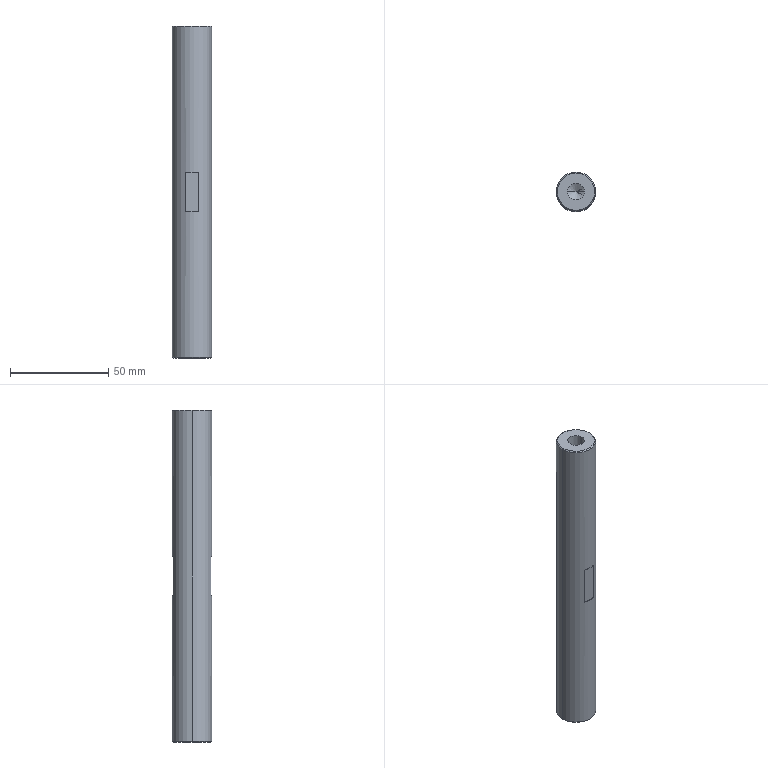Part | STEP file | 11-FG-Z01011 | 1 solid | 22 faces | box 20 x 20 x 169 mm | volume 50117 mm3 | cone 8 | plane 8 | cylinder 6 | commonest cylinder face diameters 8.5 x4 20 x2
STEP:
#1=CARTESIAN_POINT('',(-9.5,0.,0.));
#2=VERTEX_POINT('',#1);
#3=CARTESIAN_POINT('',(9.5,0.,0.));
#4=VERTEX_POINT('',#3);
#5=CARTESIAN_POINT('',(0.,0.,0.));
#6=DIRECTION('',(0.,0.,-1.));
#7=DIRECTION('',(1.,0.,0.));
#8=AXIS2_PLACEMENT_3D('',#5,#6,#7);
#9=CIRCLE('',#8,9.5);
#10=EDGE_CURVE('',#2,#4,#9,.T.);
#11=ORIENTED_EDGE('',*,*,#10,.F.);
#12=CARTESIAN_POINT('',(-10.,0.,0.5));
#13=VERTEX_POINT('',#12);
#14=CARTESIAN_POINT('',(-10.,0.,0.5));
#15=DIRECTION('',(-0.7071,0.,0.7071));
#16=VECTOR('',#15,1000.);
#17=LINE('',#14,#16);
#18=EDGE_CURVE('',#2,#13,#17,.T.);
#19=ORIENTED_EDGE('',*,*,#18,.T.);
#20=CARTESIAN_POINT('',(10.,0.,0.5));
#21=VERTEX_POINT('',#20);
#22=CARTESIAN_POINT('',(0.,0.,0.5));
#23=DIRECTION('',(0.,0.,1.));
#24=DIRECTION('',(1.,0.,0.));
#25=AXIS2_PLACEMENT_3D('',#22,#23,#24);
#26=CIRCLE('',#25,10.);
#27=EDGE_CURVE('',#21,#13,#26,.T.);
#28=ORIENTED_EDGE('',*,*,#27,.F.);
#29=CARTESIAN_POINT('',(10.,0.,0.5));
#30=DIRECTION('',(0.7071,0.,0.7071));
#31=VECTOR('',#30,1000.);
#32=LINE('',#29,#31);
#33=EDGE_CURVE('',#4,#21,#32,.T.);
#34=ORIENTED_EDGE('',*,*,#33,.F.);
#35=EDGE_LOOP('',(#11,#19,#28,#34));
#36=FACE_OUTER_BOUND('',#35,.T.);
#37=CARTESIAN_POINT('',(0.,0.,0.5));
#38=DIRECTION('',(0.,0.,1.));
#39=DIRECTION('',(1.,0.,0.));
#40=AXIS2_PLACEMENT_3D('',#37,#38,#39);
#41=CONICAL_SURFACE('',#40,10.,0.7854);
#42=ADVANCED_FACE('',(#36),#41,.T.);
#43=CARTESIAN_POINT('',(9.5,0.,169.));
#44=VERTEX_POINT('',#43);
#45=CARTESIAN_POINT('',(-9.5,0.,169.));
#46=VERTEX_POINT('',#45);
#47=CARTESIAN_POINT('',(0.,0.,169.));
#48=DIRECTION('',(0.,0.,1.));
#49=DIRECTION('',(1.,0.,0.));
#50=AXIS2_PLACEMENT_3D('',#47,#48,#49);
#51=CIRCLE('',#50,9.5);
#52=EDGE_CURVE('',#44,#46,#51,.T.);
#53=ORIENTED_EDGE('',*,*,#52,.F.);
#54=CARTESIAN_POINT('',(10.,0.,168.5));
#55=VERTEX_POINT('',#54);
#56=CARTESIAN_POINT('',(9.5,0.,169.));
#57=DIRECTION('',(0.7071,0.,-0.7071));
#58=VECTOR('',#57,1000.);
#59=LINE('',#56,#58);
#60=EDGE_CURVE('',#44,#55,#59,.T.);
#61=ORIENTED_EDGE('',*,*,#60,.T.);
#62=CARTESIAN_POINT('',(-10.,0.,168.5));
#63=VERTEX_POINT('',#62);
#64=CARTESIAN_POINT('',(0.,0.,168.5));
#65=DIRECTION('',(0.,0.,-1.));
#66=DIRECTION('',(1.,0.,0.));
#67=AXIS2_PLACEMENT_3D('',#64,#65,#66);
#68=CIRCLE('',#67,10.);
#69=EDGE_CURVE('',#63,#55,#68,.T.);
#70=ORIENTED_EDGE('',*,*,#69,.F.);
#71=CARTESIAN_POINT('',(-9.5,0.,169.));
#72=DIRECTION('',(-0.7071,0.,-0.7071));
#73=VECTOR('',#72,1000.);
#74=LINE('',#71,#73);
#75=EDGE_CURVE('',#46,#63,#74,.T.);
#76=ORIENTED_EDGE('',*,*,#75,.F.);
#77=EDGE_LOOP('',(#53,#61,#70,#76));
#78=FACE_OUTER_BOUND('',#77,.T.);
#79=CARTESIAN_POINT('',(0.,0.,169.));
#80=DIRECTION('',(0.,0.,-1.));
#81=DIRECTION('',(-1.,0.,0.));
#82=AXIS2_PLACEMENT_3D('',#79,#80,#81);
#83=CONICAL_SURFACE('',#82,9.5,0.7854);
#84=ADVANCED_FACE('',(#78),#83,.T.);
#85=CARTESIAN_POINT('',(4.25,0.,24.5));
#86=VERTEX_POINT('',#85);
#87=CARTESIAN_POINT('',(-4.25,0.,24.5));
#88=VERTEX_POINT('',#87);
#89=CARTESIAN_POINT('',(0.,0.,24.5));
#90=DIRECTION('',(0.,0.,-1.));
#91=DIRECTION('',(-1.,0.,0.));
#92=AXIS2_PLACEMENT_3D('',#89,#90,#91);
#93=CIRCLE('',#92,4.25);
#94=EDGE_CURVE('',#86,#88,#93,.T.);
#95=ORIENTED_EDGE('',*,*,#94,.F.);
#96=CARTESIAN_POINT('',(4.25,0.,0.));
#97=VERTEX_POINT('',#96);
#98=CARTESIAN_POINT('',(4.25,0.,0.));
#99=DIRECTION('',(0.,0.,-1.));
#100=VECTOR('',#99,1000.);
#101=LINE('',#98,#100);
#102=EDGE_CURVE('',#86,#97,#101,.T.);
#103=ORIENTED_EDGE('',*,*,#102,.T.);
#104=CARTESIAN_POINT('',(-4.25,0.,0.));
#105=VERTEX_POINT('',#104);
#106=CARTESIAN_POINT('',(0.,0.,0.));
#107=DIRECTION('',(0.,0.,-1.));
#108=DIRECTION('',(-1.,0.,0.));
#109=AXIS2_PLACEMENT_3D('',#106,#107,#108);
#110=CIRCLE('',#109,4.25);
#111=EDGE_CURVE('',#97,#105,#110,.T.);
#112=ORIENTED_EDGE('',*,*,#111,.T.);
#113=CARTESIAN_POINT('',(-4.25,0.,0.));
#114=DIRECTION('',(0.,0.,-1.));
#115=VECTOR('',#114,1000.);
#116=LINE('',#113,#115);
#117=EDGE_CURVE('',#88,#105,#116,.T.);
#118=ORIENTED_EDGE('',*,*,#117,.F.);
#119=EDGE_LOOP('',(#95,#103,#112,#118));
#120=FACE_OUTER_BOUND('',#119,.T.);
#121=CARTESIAN_POINT('',(0.,0.,0.));
#122=DIRECTION('',(0.,0.,-1.));
#123=DIRECTION('',(-1.,0.,0.));
#124=AXIS2_PLACEMENT_3D('',#121,#122,#123);
#125=CYLINDRICAL_SURFACE('',#124,4.25);
#126=ADVANCED_FACE('',(#120),#125,.F.);
#127=CARTESIAN_POINT('',(0.,0.,27.054));
#128=VERTEX_POINT('',#127);
#129=CARTESIAN_POINT('',(-4.25,0.,24.5));
#130=DIRECTION('',(-0.8572,0.,-0.515));
#131=VECTOR('',#130,1000.);
#132=LINE('',#129,#131);
#133=EDGE_CURVE('',#128,#88,#132,.T.);
#134=ORIENTED_EDGE('',*,*,#133,.F.);
#135=CARTESIAN_POINT('',(4.25,0.,24.5));
#136=DIRECTION('',(0.8572,0.,-0.515));
#137=VECTOR('',#136,1000.);
#138=LINE('',#135,#137);
#139=EDGE_CURVE('',#128,#86,#138,.T.);
#140=ORIENTED_EDGE('',*,*,#139,.T.);
#141=ORIENTED_EDGE('',*,*,#94,.T.);
#142=EDGE_LOOP('',(#134,#140,#141));
#143=FACE_OUTER_BOUND('',#142,.T.);
#144=CARTESIAN_POINT('',(0.,0.,24.5));
#145=DIRECTION('',(0.,0.,-1.));
#146=DIRECTION('',(-1.,0.,0.));
#147=AXIS2_PLACEMENT_3D('',#144,#145,#146);
#148=CONICAL_SURFACE('',#147,4.25,1.03);
#149=ADVANCED_FACE('',(#143),#148,.F.);
#150=CARTESIAN_POINT('',(-4.25,0.,144.5));
#151=VERTEX_POINT('',#150);
#152=CARTESIAN_POINT('',(4.25,0.,144.5));
#153=VERTEX_POINT('',#152);
#154=CARTESIAN_POINT('',(0.,0.,144.5));
#155=DIRECTION('',(0.,0.,1.));
#156=DIRECTION('',(1.,0.,0.));
#157=AXIS2_PLACEMENT_3D('',#154,#155,#156);
#158=CIRCLE('',#157,4.25);
#159=EDGE_CURVE('',#151,#153,#158,.T.);
#160=ORIENTED_EDGE('',*,*,#159,.F.);
#161=CARTESIAN_POINT('',(-4.25,0.,169.));
#162=VERTEX_POINT('',#161);
#163=CARTESIAN_POINT('',(-4.25,0.,169.));
#164=DIRECTION('',(0.,0.,1.));
#165=VECTOR('',#164,1000.);
#166=LINE('',#163,#165);
#167=EDGE_CURVE('',#151,#162,#166,.T.);
#168=ORIENTED_EDGE('',*,*,#167,.T.);
#169=CARTESIAN_POINT('',(4.25,0.,169.));
#170=VERTEX_POINT('',#169);
#171=CARTESIAN_POINT('',(0.,0.,169.));
#172=DIRECTION('',(0.,0.,1.));
#173=DIRECTION('',(1.,0.,0.));
#174=AXIS2_PLACEMENT_3D('',#171,#172,#173);
#175=CIRCLE('',#174,4.25);
#176=EDGE_CURVE('',#162,#170,#175,.T.);
#177=ORIENTED_EDGE('',*,*,#176,.T.);
#178=CARTESIAN_POINT('',(4.25,0.,169.));
#179=DIRECTION('',(0.,0.,1.));
#180=VECTOR('',#179,1000.);
#181=LINE('',#178,#180);
#182=EDGE_CURVE('',#153,#170,#181,.T.);
#183=ORIENTED_EDGE('',*,*,#182,.F.);
#184=EDGE_LOOP('',(#160,#168,#177,#183));
#185=FACE_OUTER_BOUND('',#184,.T.);
#186=CARTESIAN_POINT('',(0.,0.,169.));
#187=DIRECTION('',(0.,0.,1.));
#188=DIRECTION('',(1.,0.,0.));
#189=AXIS2_PLACEMENT_3D('',#186,#187,#188);
#190=CYLINDRICAL_SURFACE('',#189,4.25);
#191=ADVANCED_FACE('',(#185),#190,.F.);
#192=CARTESIAN_POINT('',(0.,0.,141.946));
#193=VERTEX_POINT('',#192);
#194=CARTESIAN_POINT('',(4.25,0.,144.5));
#195=DIRECTION('',(0.8572,0.,0.515));
#196=VECTOR('',#195,1000.);
#197=LINE('',#194,#196);
#198=EDGE_CURVE('',#193,#153,#197,.T.);
#199=ORIENTED_EDGE('',*,*,#198,.F.);
#200=CARTESIAN_POINT('',(-4.25,0.,144.5));
#201=DIRECTION('',(-0.8572,0.,0.515));
#202=VECTOR('',#201,1000.);
#203=LINE('',#200,#202);
#204=EDGE_CURVE('',#193,#151,#203,.T.);
#205=ORIENTED_EDGE('',*,*,#204,.T.);
#206=ORIENTED_EDGE('',*,*,#159,.T.);
#207=EDGE_LOOP('',(#199,#205,#206));
#208=FACE_OUTER_BOUND('',#207,.T.);
#209=CARTESIAN_POINT('',(0.,0.,144.5));
#210=DIRECTION('',(0.,0.,1.));
#211=DIRECTION('',(1.,0.,0.));
#212=AXIS2_PLACEMENT_3D('',#209,#210,#211);
#213=CONICAL_SURFACE('',#212,4.25,1.03);
#214=ADVANCED_FACE('',(#208),#213,.F.);
#215=CARTESIAN_POINT('',(-3.122,9.5,94.5));
#216=VERTEX_POINT('',#215);
#217=CARTESIAN_POINT('',(3.122,9.5,94.5));
#218=VERTEX_POINT('',#217);
#219=CARTESIAN_POINT('',(0.,0.,94.5));
#220=DIRECTION('',(0.,0.,-1.));
#221=DIRECTION('',(-1.,0.,0.));
#222=AXIS2_PLACEMENT_3D('',#219,#220,#221);
#223=CIRCLE('',#222,10.);
#224=EDGE_CURVE('',#216,#218,#223,.T.);
#225=ORIENTED_EDGE('',*,*,#224,.F.);
#226=CARTESIAN_POINT('',(-3.122,9.5,74.5));
#227=VERTEX_POINT('',#226);
#228=CARTESIAN_POINT('',(-3.122,9.5,169.));
#229=DIRECTION('',(0.,0.,-1.));
#230=VECTOR('',#229,1000.);
#231=LINE('',#228,#230);
#232=EDGE_CURVE('',#216,#227,#231,.T.);
#233=ORIENTED_EDGE('',*,*,#232,.T.);
#234=CARTESIAN_POINT('',(3.122,9.5,74.5));
#235=VERTEX_POINT('',#234);
#236=CARTESIAN_POINT('',(0.,0.,74.5));
#237=DIRECTION('',(0.,0.,-1.));
#238=DIRECTION('',(-1.,0.,0.));
#239=AXIS2_PLACEMENT_3D('',#236,#237,#238);
#240=CIRCLE('',#239,10.);
#241=EDGE_CURVE('',#227,#235,#240,.T.);
#242=ORIENTED_EDGE('',*,*,#241,.T.);
#243=CARTESIAN_POINT('',(3.122,9.5,169.));
#244=DIRECTION('',(0.,0.,1.));
#245=VECTOR('',#244,1000.);
#246=LINE('',#243,#245);
#247=EDGE_CURVE('',#235,#218,#246,.T.);
#248=ORIENTED_EDGE('',*,*,#247,.T.);
#249=EDGE_LOOP('',(#225,#233,#242,#248));
#250=FACE_BOUND('',#249,.T.);
#251=ORIENTED_EDGE('',*,*,#69,.T.);
#252=CARTESIAN_POINT('',(10.,0.,169.));
#253=DIRECTION('',(0.,0.,-1.));
#254=VECTOR('',#253,1000.);
#255=LINE('',#252,#254);
#256=EDGE_CURVE('',#55,#21,#255,.T.);
#257=ORIENTED_EDGE('',*,*,#256,.T.);
#258=ORIENTED_EDGE('',*,*,#27,.T.);
#259=CARTESIAN_POINT('',(-10.,0.,169.));
#260=DIRECTION('',(0.,0.,-1.));
#261=VECTOR('',#260,1000.);
#262=LINE('',#259,#261);
#263=EDGE_CURVE('',#63,#13,#262,.T.);
#264=ORIENTED_EDGE('',*,*,#263,.F.);
#265=EDGE_LOOP('',(#251,#257,#258,#264));
#266=FACE_OUTER_BOUND('',#265,.T.);
#267=CARTESIAN_POINT('',(0.,0.,169.));
#268=DIRECTION('',(0.,0.,-1.));
#269=DIRECTION('',(-1.,0.,0.));
#270=AXIS2_PLACEMENT_3D('',#267,#268,#269);
#271=CYLINDRICAL_SURFACE('',#270,10.);
#272=ADVANCED_FACE('',(#250,#266),#271,.T.);
#273=ORIENTED_EDGE('',*,*,#256,.F.);
#274=CARTESIAN_POINT('',(0.,0.,168.5));
#275=DIRECTION('',(0.,0.,-1.));
#276=DIRECTION('',(1.,0.,0.));
#277=AXIS2_PLACEMENT_3D('',#274,#275,#276);
#278=CIRCLE('',#277,10.);
#279=EDGE_CURVE('',#55,#63,#278,.T.);
#280=ORIENTED_EDGE('',*,*,#279,.T.);
#281=ORIENTED_EDGE('',*,*,#263,.T.);
#282=CARTESIAN_POINT('',(0.,0.,0.5));
#283=DIRECTION('',(0.,0.,1.));
#284=DIRECTION('',(1.,0.,0.));
#285=AXIS2_PLACEMENT_3D('',#282,#283,#284);
#286=CIRCLE('',#285,10.);
#287=EDGE_CURVE('',#13,#21,#286,.T.);
#288=ORIENTED_EDGE('',*,*,#287,.T.);
#289=EDGE_LOOP('',(#273,#280,#281,#288));
#290=FACE_OUTER_BOUND('',#289,.T.);
#291=CARTESIAN_POINT('',(3.122,-9.5,94.5));
#292=VERTEX_POINT('',#291);
#293=CARTESIAN_POINT('',(-3.122,-9.5,94.5));
#294=VERTEX_POINT('',#293);
#295=CARTESIAN_POINT('',(0.,0.,94.5));
#296=DIRECTION('',(0.,0.,-1.));
#297=DIRECTION('',(-1.,0.,0.));
#298=AXIS2_PLACEMENT_3D('',#295,#296,#297);
#299=CIRCLE('',#298,10.);
#300=EDGE_CURVE('',#292,#294,#299,.T.);
#301=ORIENTED_EDGE('',*,*,#300,.F.);
#302=CARTESIAN_POINT('',(3.122,-9.5,74.5));
#303=VERTEX_POINT('',#302);
#304=CARTESIAN_POINT('',(3.122,-9.5,169.));
#305=DIRECTION('',(0.,0.,-1.));
#306=VECTOR('',#305,1000.);
#307=LINE('',#304,#306);
#308=EDGE_CURVE('',#292,#303,#307,.T.);
#309=ORIENTED_EDGE('',*,*,#308,.T.);
#310=CARTESIAN_POINT('',(-3.122,-9.5,74.5));
#311=VERTEX_POINT('',#310);
#312=CARTESIAN_POINT('',(0.,0.,74.5));
#313=DIRECTION('',(0.,0.,-1.));
#314=DIRECTION('',(-1.,0.,0.));
#315=AXIS2_PLACEMENT_3D('',#312,#313,#314);
#316=CIRCLE('',#315,10.);
#317=EDGE_CURVE('',#303,#311,#316,.T.);
#318=ORIENTED_EDGE('',*,*,#317,.T.);
#319=CARTESIAN_POINT('',(-3.122,-9.5,169.));
#320=DIRECTION('',(0.,0.,1.));
#321=VECTOR('',#320,1000.);
#322=LINE('',#319,#321);
#323=EDGE_CURVE('',#311,#294,#322,.T.);
#324=ORIENTED_EDGE('',*,*,#323,.T.);
#325=EDGE_LOOP('',(#301,#309,#318,#324));
#326=FACE_BOUND('',#325,.T.);
#327=CARTESIAN_POINT('',(0.,0.,169.));
#328=DIRECTION('',(0.,0.,-1.));
#329=DIRECTION('',(-1.,0.,0.));
#330=AXIS2_PLACEMENT_3D('',#327,#328,#329);
#331=CYLINDRICAL_SURFACE('',#330,10.);
#332=ADVANCED_FACE('',(#290,#326),#331,.T.);
#333=CARTESIAN_POINT('',(0.,0.,169.));
#334=DIRECTION('',(0.,0.,1.));
#335=DIRECTION('',(1.,0.,0.));
#336=AXIS2_PLACEMENT_3D('',#333,#334,#335);
#337=CIRCLE('',#336,9.5);
#338=EDGE_CURVE('',#46,#44,#337,.T.);
#339=ORIENTED_EDGE('',*,*,#338,.T.);
#340=ORIENTED_EDGE('',*,*,#52,.T.);
#341=EDGE_LOOP('',(#339,#340));
#342=FACE_OUTER_BOUND('',#341,.T.);
#343=CARTESIAN_POINT('',(0.,0.,169.));
#344=DIRECTION('',(0.,0.,1.));
#345=DIRECTION('',(1.,0.,0.));
#346=AXIS2_PLACEMENT_3D('',#343,#344,#345);
#347=CIRCLE('',#346,4.25);
#348=EDGE_CURVE('',#170,#162,#347,.T.);
#349=ORIENTED_EDGE('',*,*,#348,.F.);
#350=ORIENTED_EDGE('',*,*,#176,.F.);
#351=EDGE_LOOP('',(#349,#350));
#352=FACE_BOUND('',#351,.T.);
#353=CARTESIAN_POINT('',(0.,0.,169.));
#354=DIRECTION('',(0.,0.,1.));
#355=DIRECTION('',(1.,0.,0.));
#356=AXIS2_PLACEMENT_3D('',#353,#354,#355);
#357=PLANE('',#356);
#358=ADVANCED_FACE('',(#342,#352),#357,.T.);
#359=CARTESIAN_POINT('',(0.,0.,0.));
#360=DIRECTION('',(0.,0.,-1.));
#361=DIRECTION('',(1.,0.,0.));
#362=AXIS2_PLACEMENT_3D('',#359,#360,#361);
#363=CIRCLE('',#362,9.5);
#364=EDGE_CURVE('',#4,#2,#363,.T.);
#365=ORIENTED_EDGE('',*,*,#364,.T.);
#366=ORIENTED_EDGE('',*,*,#10,.T.);
#367=EDGE_LOOP('',(#365,#366));
#368=FACE_OUTER_BOUND('',#367,.T.);
#369=CARTESIAN_POINT('',(0.,0.,0.));
#370=DIRECTION('',(0.,0.,-1.));
#371=DIRECTION('',(-1.,0.,0.));
#372=AXIS2_PLACEMENT_3D('',#369,#370,#371);
#373=CIRCLE('',#372,4.25);
#374=EDGE_CURVE('',#105,#97,#373,.T.);
#375=ORIENTED_EDGE('',*,*,#374,.F.);
#376=ORIENTED_EDGE('',*,*,#111,.F.);
#377=EDGE_LOOP('',(#375,#376));
#378=FACE_BOUND('',#377,.T.);
#379=CARTESIAN_POINT('',(0.,0.,0.));
#380=DIRECTION('',(0.,0.,1.));
#381=DIRECTION('',(1.,0.,0.));
#382=AXIS2_PLACEMENT_3D('',#379,#380,#381);
#383=PLANE('',#382);
#384=ADVANCED_FACE('',(#368,#378),#383,.F.);
#385=ORIENTED_EDGE('',*,*,#204,.F.);
#386=ORIENTED_EDGE('',*,*,#198,.T.);
#387=CARTESIAN_POINT('',(0.,0.,144.5));
#388=DIRECTION('',(0.,0.,1.));
#389=DIRECTION('',(1.,0.,0.));
#390=AXIS2_PLACEMENT_3D('',#387,#388,#389);
#391=CIRCLE('',#390,4.25);
#392=EDGE_CURVE('',#153,#151,#391,.T.);
#393=ORIENTED_EDGE('',*,*,#392,.T.);
#394=EDGE_LOOP('',(#385,#386,#393));
#395=FACE_OUTER_BOUND('',#394,.T.);
#396=CARTESIAN_POINT('',(0.,0.,144.5));
#397=DIRECTION('',(0.,0.,1.));
#398=DIRECTION('',(1.,0.,0.));
#399=AXIS2_PLACEMENT_3D('',#396,#397,#398);
#400=CONICAL_SURFACE('',#399,4.25,1.03);
#401=ADVANCED_FACE('',(#395),#400,.F.);
#402=ORIENTED_EDGE('',*,*,#167,.F.);
#403=ORIENTED_EDGE('',*,*,#392,.F.);
#404=ORIENTED_EDGE('',*,*,#182,.T.);
#405=ORIENTED_EDGE('',*,*,#348,.T.);
#406=EDGE_LOOP('',(#402,#403,#404,#405));
#407=FACE_OUTER_BOUND('',#406,.T.);
#408=CARTESIAN_POINT('',(0.,0.,169.));
#409=DIRECTION('',(0.,0.,1.));
#410=DIRECTION('',(1.,0.,0.));
#411=AXIS2_PLACEMENT_3D('',#408,#409,#410);
#412=CYLINDRICAL_SURFACE('',#411,4.25);
#413=ADVANCED_FACE('',(#407),#412,.F.);
#414=ORIENTED_EDGE('',*,*,#139,.F.);
#415=ORIENTED_EDGE('',*,*,#133,.T.);
#416=CARTESIAN_POINT('',(0.,0.,24.5));
#417=DIRECTION('',(0.,0.,-1.));
#418=DIRECTION('',(-1.,0.,0.));
#419=AXIS2_PLACEMENT_3D('',#416,#417,#418);
#420=CIRCLE('',#419,4.25);
#421=EDGE_CURVE('',#88,#86,#420,.T.);
#422=ORIENTED_EDGE('',*,*,#421,.T.);
#423=EDGE_LOOP('',(#414,#415,#422));
#424=FACE_OUTER_BOUND('',#423,.T.);
#425=CARTESIAN_POINT('',(0.,0.,24.5));
#426=DIRECTION('',(0.,0.,-1.));
#427=DIRECTION('',(-1.,0.,0.));
#428=AXIS2_PLACEMENT_3D('',#425,#426,#427);
#429=CONICAL_SURFACE('',#428,4.25,1.03);
#430=ADVANCED_FACE('',(#424),#429,.F.);
#431=ORIENTED_EDGE('',*,*,#102,.F.);
#432=ORIENTED_EDGE('',*,*,#421,.F.);
#433=ORIENTED_EDGE('',*,*,#117,.T.);
#434=ORIENTED_EDGE('',*,*,#374,.T.);
#435=EDGE_LOOP('',(#431,#432,#433,#434));
#436=FACE_OUTER_BOUND('',#435,.T.);
#437=CARTESIAN_POINT('',(0.,0.,0.));
#438=DIRECTION('',(0.,0.,-1.));
#439=DIRECTION('',(-1.,0.,0.));
#440=AXIS2_PLACEMENT_3D('',#437,#438,#439);
#441=CYLINDRICAL_SURFACE('',#440,4.25);
#442=ADVANCED_FACE('',(#436),#441,.F.);
#443=ORIENTED_EDGE('',*,*,#60,.F.);
#444=ORIENTED_EDGE('',*,*,#338,.F.);
#445=ORIENTED_EDGE('',*,*,#75,.T.);
#446=ORIENTED_EDGE('',*,*,#279,.F.);
#447=EDGE_LOOP('',(#443,#444,#445,#446));
#448=FACE_OUTER_BOUND('',#447,.T.);
#449=CARTESIAN_POINT('',(0.,0.,169.));
#450=DIRECTION('',(0.,0.,-1.));
#451=DIRECTION('',(-1.,0.,0.));
#452=AXIS2_PLACEMENT_3D('',#449,#450,#451);
#453=CONICAL_SURFACE('',#452,9.5,0.7854);
#454=ADVANCED_FACE('',(#448),#453,.T.);
#455=ORIENTED_EDGE('',*,*,#18,.F.);
#456=ORIENTED_EDGE('',*,*,#364,.F.);
#457=ORIENTED_EDGE('',*,*,#33,.T.);
#458=ORIENTED_EDGE('',*,*,#287,.F.);
#459=EDGE_LOOP('',(#455,#456,#457,#458));
#460=FACE_OUTER_BOUND('',#459,.T.);
#461=CARTESIAN_POINT('',(0.,0.,0.5));
#462=DIRECTION('',(0.,0.,1.));
#463=DIRECTION('',(1.,0.,0.));
#464=AXIS2_PLACEMENT_3D('',#461,#462,#463);
#465=CONICAL_SURFACE('',#464,10.,0.7854);
#466=ADVANCED_FACE('',(#460),#465,.T.);
#467=CARTESIAN_POINT('',(4.899,9.5,94.5));
#468=DIRECTION('',(-1.,0.,0.));
#469=VECTOR('',#468,1000.);
#470=LINE('',#467,#469);
#471=EDGE_CURVE('',#218,#216,#470,.T.);
#472=ORIENTED_EDGE('',*,*,#471,.F.);
#473=ORIENTED_EDGE('',*,*,#247,.F.);
#474=CARTESIAN_POINT('',(4.899,9.5,74.5));
#475=DIRECTION('',(-1.,0.,0.));
#476=VECTOR('',#475,1000.);
#477=LINE('',#474,#476);
#478=EDGE_CURVE('',#235,#227,#477,.T.);
#479=ORIENTED_EDGE('',*,*,#478,.T.);
#480=ORIENTED_EDGE('',*,*,#232,.F.);
#481=EDGE_LOOP('',(#472,#473,#479,#480));
#482=FACE_OUTER_BOUND('',#481,.T.);
#483=CARTESIAN_POINT('',(4.899,9.5,94.5));
#484=DIRECTION('',(0.,-1.,0.));
#485=DIRECTION('',(0.,0.,-1.));
#486=AXIS2_PLACEMENT_3D('',#483,#484,#485);
#487=PLANE('',#486);
#488=ADVANCED_FACE('',(#482),#487,.F.);
#489=ORIENTED_EDGE('',*,*,#224,.T.);
#490=ORIENTED_EDGE('',*,*,#471,.T.);
#491=EDGE_LOOP('',(#489,#490));
#492=FACE_OUTER_BOUND('',#491,.T.);
#493=CARTESIAN_POINT('',(0.,0.,94.5));
#494=DIRECTION('',(0.,0.,-1.));
#495=DIRECTION('',(-1.,0.,0.));
#496=AXIS2_PLACEMENT_3D('',#493,#494,#495);
#497=PLANE('',#496);
#498=ADVANCED_FACE('',(#492),#497,.T.);
#499=ORIENTED_EDGE('',*,*,#478,.F.);
#500=ORIENTED_EDGE('',*,*,#241,.F.);
#501=EDGE_LOOP('',(#499,#500));
#502=FACE_OUTER_BOUND('',#501,.T.);
#503=CARTESIAN_POINT('',(0.,0.,74.5));
#504=DIRECTION('',(0.,0.,-1.));
#505=DIRECTION('',(-1.,0.,0.));
#506=AXIS2_PLACEMENT_3D('',#503,#504,#505);
#507=PLANE('',#506);
#508=ADVANCED_FACE('',(#502),#507,.F.);
#509=CARTESIAN_POINT('',(4.899,-9.5,94.5));
#510=DIRECTION('',(1.,0.,0.));
#511=VECTOR('',#510,1000.);
#512=LINE('',#509,#511);
#513=EDGE_CURVE('',#294,#292,#512,.T.);
#514=ORIENTED_EDGE('',*,*,#513,.F.);
#515=ORIENTED_EDGE('',*,*,#323,.F.);
#516=CARTESIAN_POINT('',(4.899,-9.5,74.5));
#517=DIRECTION('',(1.,0.,0.));
#518=VECTOR('',#517,1000.);
#519=LINE('',#516,#518);
#520=EDGE_CURVE('',#311,#303,#519,.T.);
#521=ORIENTED_EDGE('',*,*,#520,.T.);
#522=ORIENTED_EDGE('',*,*,#308,.F.);
#523=EDGE_LOOP('',(#514,#515,#521,#522));
#524=FACE_OUTER_BOUND('',#523,.T.);
#525=CARTESIAN_POINT('',(4.899,-9.5,94.5));
#526=DIRECTION('',(0.,1.,0.));
#527=DIRECTION('',(0.,0.,1.));
#528=AXIS2_PLACEMENT_3D('',#525,#526,#527);
#529=PLANE('',#528);
#530=ADVANCED_FACE('',(#524),#529,.F.);
#531=ORIENTED_EDGE('',*,*,#300,.T.);
#532=ORIENTED_EDGE('',*,*,#513,.T.);
#533=EDGE_LOOP('',(#531,#532));
#534=FACE_OUTER_BOUND('',#533,.T.);
#535=CARTESIAN_POINT('',(0.,0.,94.5));
#536=DIRECTION('',(0.,0.,-1.));
#537=DIRECTION('',(-1.,0.,0.));
#538=AXIS2_PLACEMENT_3D('',#535,#536,#537);
#539=PLANE('',#538);
#540=ADVANCED_FACE('',(#534),#539,.T.);
#541=ORIENTED_EDGE('',*,*,#520,.F.);
#542=ORIENTED_EDGE('',*,*,#317,.F.);
#543=EDGE_LOOP('',(#541,#542));
#544=FACE_OUTER_BOUND('',#543,.T.);
#545=CARTESIAN_POINT('',(0.,0.,74.5));
#546=DIRECTION('',(0.,0.,-1.));
#547=DIRECTION('',(-1.,0.,0.));
#548=AXIS2_PLACEMENT_3D('',#545,#546,#547);
#549=PLANE('',#548);
#550=ADVANCED_FACE('',(#544),#549,.F.);
#551=CLOSED_SHELL('',(#42,#84,#126,#149,#191,#214,#272,#332,#358,#384,#401,#413,#430,#442,#454,#466,#488,#498,#508,#530,#540,#550));
#552=MANIFOLD_SOLID_BREP('',#551);
#553=CARTESIAN_POINT('',(0.,0.,0.));
#554=DIRECTION('',(0.,0.,1.));
#555=DIRECTION('',(1.,0.,0.));
#556=AXIS2_PLACEMENT_3D('',#553,#554,#555);
#557=(LENGTH_UNIT()NAMED_UNIT(*)SI_UNIT(.MILLI.,.METRE.));
#558=UNCERTAINTY_MEASURE_WITH_UNIT(LENGTH_MEASURE(0.00001),#557,'','');
#559=(NAMED_UNIT(*)PLANE_ANGLE_UNIT()SI_UNIT($,.RADIAN.));
#560=(NAMED_UNIT(*)SI_UNIT($,.STERADIAN.)SOLID_ANGLE_UNIT());
#561=(GEOMETRIC_REPRESENTATION_CONTEXT(3)GLOBAL_UNCERTAINTY_ASSIGNED_CONTEXT((#558))GLOBAL_UNIT_ASSIGNED_CONTEXT((#557,#559,#560))REPRESENTATION_CONTEXT('',''));
#562=ADVANCED_BREP_SHAPE_REPRESENTATION('',(#552,#556),#561);